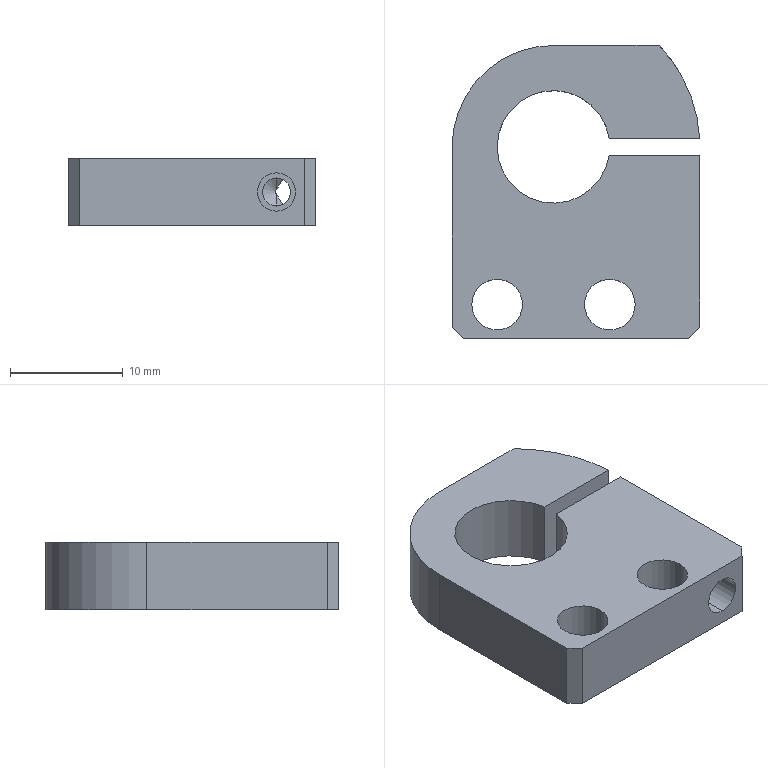Part | STEP file | FBDS-CS-020 | 1 solid | 25 faces | box 22 x 26 x 6 mm | volume 2342 mm3 | cylinder 12 | plane 10 | cone 3 | commonest cylinder face diameters 4.5 x4 2.5 x2 3.4 x2 10 x2 18 x1 26 x1
STEP:
#1=CARTESIAN_POINT('',(-581.954,-3556.136,6.));
#2=VERTEX_POINT('',#1);
#3=CARTESIAN_POINT('',(-577.454,-3556.136,6.));
#4=VERTEX_POINT('',#3);
#5=CARTESIAN_POINT('',(-579.704,-3556.136,6.));
#6=DIRECTION('',(0.,0.,1.));
#7=DIRECTION('',(1.,0.,0.));
#8=AXIS2_PLACEMENT_3D('',#5,#6,#7);
#9=CIRCLE('',#8,2.25);
#10=EDGE_CURVE('',#2,#4,#9,.T.);
#11=ORIENTED_EDGE('',*,*,#10,.T.);
#12=CARTESIAN_POINT('',(-577.454,-3556.136,0.));
#13=VERTEX_POINT('',#12);
#14=CARTESIAN_POINT('',(-577.454,-3556.136,0.));
#15=DIRECTION('',(0.,0.,-1.));
#16=VECTOR('',#15,1000.);
#17=LINE('',#14,#16);
#18=EDGE_CURVE('',#4,#13,#17,.T.);
#19=ORIENTED_EDGE('',*,*,#18,.T.);
#20=CARTESIAN_POINT('',(-581.954,-3556.136,0.));
#21=VERTEX_POINT('',#20);
#22=CARTESIAN_POINT('',(-579.704,-3556.136,0.));
#23=DIRECTION('',(0.,0.,-1.));
#24=DIRECTION('',(-1.,0.,0.));
#25=AXIS2_PLACEMENT_3D('',#22,#23,#24);
#26=CIRCLE('',#25,2.25);
#27=EDGE_CURVE('',#13,#21,#26,.T.);
#28=ORIENTED_EDGE('',*,*,#27,.T.);
#29=CARTESIAN_POINT('',(-581.954,-3556.136,0.));
#30=DIRECTION('',(0.,0.,-1.));
#31=VECTOR('',#30,1000.);
#32=LINE('',#29,#31);
#33=EDGE_CURVE('',#2,#21,#32,.T.);
#34=ORIENTED_EDGE('',*,*,#33,.F.);
#35=EDGE_LOOP('',(#11,#19,#28,#34));
#36=FACE_OUTER_BOUND('',#35,.T.);
#37=CARTESIAN_POINT('',(-579.704,-3556.136,0.));
#38=DIRECTION('',(0.,0.,-1.));
#39=DIRECTION('',(-1.,0.,0.));
#40=AXIS2_PLACEMENT_3D('',#37,#38,#39);
#41=CYLINDRICAL_SURFACE('',#40,2.25);
#42=ADVANCED_FACE('',(#36),#41,.F.);
#43=CARTESIAN_POINT('',(-591.954,-3556.136,6.));
#44=VERTEX_POINT('',#43);
#45=CARTESIAN_POINT('',(-587.454,-3556.136,6.));
#46=VERTEX_POINT('',#45);
#47=CARTESIAN_POINT('',(-589.704,-3556.136,6.));
#48=DIRECTION('',(0.,0.,1.));
#49=DIRECTION('',(1.,0.,0.));
#50=AXIS2_PLACEMENT_3D('',#47,#48,#49);
#51=CIRCLE('',#50,2.25);
#52=EDGE_CURVE('',#44,#46,#51,.T.);
#53=ORIENTED_EDGE('',*,*,#52,.T.);
#54=CARTESIAN_POINT('',(-587.454,-3556.136,0.));
#55=VERTEX_POINT('',#54);
#56=CARTESIAN_POINT('',(-587.454,-3556.136,0.));
#57=DIRECTION('',(0.,0.,-1.));
#58=VECTOR('',#57,1000.);
#59=LINE('',#56,#58);
#60=EDGE_CURVE('',#46,#55,#59,.T.);
#61=ORIENTED_EDGE('',*,*,#60,.T.);
#62=CARTESIAN_POINT('',(-591.954,-3556.136,0.));
#63=VERTEX_POINT('',#62);
#64=CARTESIAN_POINT('',(-589.704,-3556.136,0.));
#65=DIRECTION('',(0.,0.,-1.));
#66=DIRECTION('',(-1.,0.,0.));
#67=AXIS2_PLACEMENT_3D('',#64,#65,#66);
#68=CIRCLE('',#67,2.25);
#69=EDGE_CURVE('',#55,#63,#68,.T.);
#70=ORIENTED_EDGE('',*,*,#69,.T.);
#71=CARTESIAN_POINT('',(-591.954,-3556.136,0.));
#72=DIRECTION('',(0.,0.,-1.));
#73=VECTOR('',#72,1000.);
#74=LINE('',#71,#73);
#75=EDGE_CURVE('',#44,#63,#74,.T.);
#76=ORIENTED_EDGE('',*,*,#75,.F.);
#77=EDGE_LOOP('',(#53,#61,#70,#76));
#78=FACE_OUTER_BOUND('',#77,.T.);
#79=CARTESIAN_POINT('',(-589.704,-3556.136,0.));
#80=DIRECTION('',(0.,0.,-1.));
#81=DIRECTION('',(-1.,0.,0.));
#82=AXIS2_PLACEMENT_3D('',#79,#80,#81);
#83=CYLINDRICAL_SURFACE('',#82,2.25);
#84=ADVANCED_FACE('',(#78),#83,.F.);
#85=CARTESIAN_POINT('',(-575.204,-3533.262,3.211));
#86=VERTEX_POINT('',#85);
#87=CARTESIAN_POINT('',(-575.204,-3533.262,2.789));
#88=VERTEX_POINT('',#87);
#89=CARTESIAN_POINT('',(-575.204,-3533.262,3.211));
#90=CARTESIAN_POINT('',(-575.222,-3533.243,3.18));
#91=CARTESIAN_POINT('',(-575.239,-3533.225,3.148));
#92=CARTESIAN_POINT('',(-575.268,-3533.194,3.079));
#93=CARTESIAN_POINT('',(-575.28,-3533.181,3.04));
#94=CARTESIAN_POINT('',(-575.28,-3533.181,2.959));
#95=CARTESIAN_POINT('',(-575.268,-3533.194,2.92));
#96=CARTESIAN_POINT('',(-575.238,-3533.225,2.851));
#97=CARTESIAN_POINT('',(-575.221,-3533.243,2.82));
#98=CARTESIAN_POINT('',(-575.204,-3533.262,2.789));
#99=B_SPLINE_CURVE_WITH_KNOTS('',3,(#89,#90,#91,#92,#93,#94,#95,#96,#97,#98),.UNSPECIFIED.,.F.,.F.,(4,2,2,2,4),(0.00138,0.001502,0.001624,0.001746,0.001868),.UNSPECIFIED.);
#100=EDGE_CURVE('',#86,#88,#99,.T.);
#101=ORIENTED_EDGE('',*,*,#100,.F.);
#102=CARTESIAN_POINT('',(-575.204,-3533.886,4.25));
#103=VERTEX_POINT('',#102);
#104=CARTESIAN_POINT('',(-575.204,-3533.886,4.25));
#105=DIRECTION('',(0.,-0.515,0.8572));
#106=VECTOR('',#105,1000.);
#107=LINE('',#104,#106);
#108=EDGE_CURVE('',#86,#103,#107,.T.);
#109=ORIENTED_EDGE('',*,*,#108,.T.);
#110=CARTESIAN_POINT('',(-575.204,-3533.886,1.75));
#111=VERTEX_POINT('',#110);
#112=CARTESIAN_POINT('',(-575.204,-3533.886,3.));
#113=DIRECTION('',(0.,-1.,0.));
#114=DIRECTION('',(0.,0.,-1.));
#115=AXIS2_PLACEMENT_3D('',#112,#113,#114);
#116=CIRCLE('',#115,1.25);
#117=EDGE_CURVE('',#103,#111,#116,.T.);
#118=ORIENTED_EDGE('',*,*,#117,.T.);
#119=CARTESIAN_POINT('',(-575.204,-3533.886,1.75));
#120=DIRECTION('',(0.,-0.515,-0.8572));
#121=VECTOR('',#120,1000.);
#122=LINE('',#119,#121);
#123=EDGE_CURVE('',#88,#111,#122,.T.);
#124=ORIENTED_EDGE('',*,*,#123,.F.);
#125=EDGE_LOOP('',(#101,#109,#118,#124));
#126=FACE_OUTER_BOUND('',#125,.T.);
#127=CARTESIAN_POINT('',(-575.204,-3533.886,3.));
#128=DIRECTION('',(0.,-1.,0.));
#129=DIRECTION('',(0.,0.,-1.));
#130=AXIS2_PLACEMENT_3D('',#127,#128,#129);
#131=CONICAL_SURFACE('',#130,1.25,1.03);
#132=ADVANCED_FACE('',(#126),#131,.F.);
#133=CARTESIAN_POINT('',(-574.657,-3533.886,1.876));
#134=VERTEX_POINT('',#133);
#135=CARTESIAN_POINT('',(-575.204,-3533.262,2.789));
#136=CARTESIAN_POINT('',(-575.159,-3533.31,2.709));
#137=CARTESIAN_POINT('',(-575.112,-3533.362,2.634));
#138=CARTESIAN_POINT('',(-575.018,-3533.465,2.483));
#139=CARTESIAN_POINT('',(-574.972,-3533.517,2.408));
#140=CARTESIAN_POINT('',(-574.834,-3533.675,2.181));
#141=CARTESIAN_POINT('',(-574.744,-3533.781,2.029));
#142=CARTESIAN_POINT('',(-574.657,-3533.886,1.876));
#143=B_SPLINE_CURVE_WITH_KNOTS('',3,(#135,#136,#137,#138,#139,#140,#141,#142),.UNSPECIFIED.,.F.,.F.,(4,2,2,4),(0.001868,0.002179,0.00249,0.003112),.UNSPECIFIED.);
#144=EDGE_CURVE('',#88,#134,#143,.T.);
#145=ORIENTED_EDGE('',*,*,#144,.F.);
#146=ORIENTED_EDGE('',*,*,#123,.T.);
#147=CARTESIAN_POINT('',(-575.204,-3533.886,3.));
#148=DIRECTION('',(0.,-1.,0.));
#149=DIRECTION('',(0.,0.,-1.));
#150=AXIS2_PLACEMENT_3D('',#147,#148,#149);
#151=CIRCLE('',#150,1.25);
#152=EDGE_CURVE('',#111,#134,#151,.T.);
#153=ORIENTED_EDGE('',*,*,#152,.T.);
#154=EDGE_LOOP('',(#145,#146,#153));
#155=FACE_OUTER_BOUND('',#154,.T.);
#156=CARTESIAN_POINT('',(-575.204,-3533.886,3.));
#157=DIRECTION('',(0.,-1.,0.));
#158=DIRECTION('',(0.,0.,-1.));
#159=AXIS2_PLACEMENT_3D('',#156,#157,#158);
#160=CONICAL_SURFACE('',#159,1.25,1.03);
#161=ADVANCED_FACE('',(#155),#160,.F.);
#162=ORIENTED_EDGE('',*,*,#117,.F.);
#163=CARTESIAN_POINT('',(-575.204,-3541.386,4.25));
#164=VERTEX_POINT('',#163);
#165=CARTESIAN_POINT('',(-575.204,-3541.386,4.25));
#166=DIRECTION('',(0.,-1.,0.));
#167=VECTOR('',#166,1000.);
#168=LINE('',#165,#167);
#169=EDGE_CURVE('',#103,#164,#168,.T.);
#170=ORIENTED_EDGE('',*,*,#169,.T.);
#171=CARTESIAN_POINT('',(-575.204,-3541.386,1.75));
#172=VERTEX_POINT('',#171);
#173=CARTESIAN_POINT('',(-575.204,-3541.386,3.));
#174=DIRECTION('',(0.,-1.,0.));
#175=DIRECTION('',(0.,0.,-1.));
#176=AXIS2_PLACEMENT_3D('',#173,#174,#175);
#177=CIRCLE('',#176,1.25);
#178=EDGE_CURVE('',#164,#172,#177,.T.);
#179=ORIENTED_EDGE('',*,*,#178,.T.);
#180=CARTESIAN_POINT('',(-575.204,-3541.386,1.75));
#181=DIRECTION('',(0.,-1.,0.));
#182=VECTOR('',#181,1000.);
#183=LINE('',#180,#182);
#184=EDGE_CURVE('',#111,#172,#183,.T.);
#185=ORIENTED_EDGE('',*,*,#184,.F.);
#186=EDGE_LOOP('',(#162,#170,#179,#185));
#187=FACE_OUTER_BOUND('',#186,.T.);
#188=CARTESIAN_POINT('',(-575.204,-3541.386,3.));
#189=DIRECTION('',(0.,-1.,0.));
#190=DIRECTION('',(0.,0.,-1.));
#191=AXIS2_PLACEMENT_3D('',#188,#189,#190);
#192=CYLINDRICAL_SURFACE('',#191,1.25);
#193=ADVANCED_FACE('',(#187),#192,.F.);
#194=CARTESIAN_POINT('',(-575.204,-3542.886,1.3));
#195=VERTEX_POINT('',#194);
#196=CARTESIAN_POINT('',(-575.204,-3542.886,4.7));
#197=VERTEX_POINT('',#196);
#198=CARTESIAN_POINT('',(-575.204,-3542.886,3.));
#199=DIRECTION('',(0.,1.,0.));
#200=DIRECTION('',(0.,0.,-1.));
#201=AXIS2_PLACEMENT_3D('',#198,#199,#200);
#202=CIRCLE('',#201,1.7);
#203=EDGE_CURVE('',#195,#197,#202,.T.);
#204=ORIENTED_EDGE('',*,*,#203,.T.);
#205=CARTESIAN_POINT('',(-575.204,-3559.136,4.7));
#206=VERTEX_POINT('',#205);
#207=CARTESIAN_POINT('',(-575.204,-3559.136,4.7));
#208=DIRECTION('',(0.,-1.,0.));
#209=VECTOR('',#208,1000.);
#210=LINE('',#207,#209);
#211=EDGE_CURVE('',#197,#206,#210,.T.);
#212=ORIENTED_EDGE('',*,*,#211,.T.);
#213=CARTESIAN_POINT('',(-575.204,-3559.136,1.3));
#214=VERTEX_POINT('',#213);
#215=CARTESIAN_POINT('',(-575.204,-3559.136,3.));
#216=DIRECTION('',(0.,-1.,0.));
#217=DIRECTION('',(0.,0.,-1.));
#218=AXIS2_PLACEMENT_3D('',#215,#216,#217);
#219=CIRCLE('',#218,1.7);
#220=EDGE_CURVE('',#206,#214,#219,.T.);
#221=ORIENTED_EDGE('',*,*,#220,.T.);
#222=CARTESIAN_POINT('',(-575.204,-3559.136,1.3));
#223=DIRECTION('',(0.,-1.,0.));
#224=VECTOR('',#223,1000.);
#225=LINE('',#222,#224);
#226=EDGE_CURVE('',#195,#214,#225,.T.);
#227=ORIENTED_EDGE('',*,*,#226,.F.);
#228=EDGE_LOOP('',(#204,#212,#221,#227));
#229=FACE_OUTER_BOUND('',#228,.T.);
#230=CARTESIAN_POINT('',(-575.204,-3559.136,3.));
#231=DIRECTION('',(0.,-1.,0.));
#232=DIRECTION('',(0.,0.,-1.));
#233=AXIS2_PLACEMENT_3D('',#230,#231,#232);
#234=CYLINDRICAL_SURFACE('',#233,1.7);
#235=ADVANCED_FACE('',(#229),#234,.F.);
#236=CARTESIAN_POINT('',(-579.761,-3541.386,6.));
#237=VERTEX_POINT('',#236);
#238=CARTESIAN_POINT('',(-589.704,-3542.136,6.));
#239=VERTEX_POINT('',#238);
#240=CARTESIAN_POINT('',(-584.704,-3542.136,6.));
#241=DIRECTION('',(0.,0.,1.));
#242=DIRECTION('',(1.,0.,0.));
#243=AXIS2_PLACEMENT_3D('',#240,#241,#242);
#244=CIRCLE('',#243,5.);
#245=EDGE_CURVE('',#237,#239,#244,.T.);
#246=ORIENTED_EDGE('',*,*,#245,.T.);
#247=CARTESIAN_POINT('',(-589.704,-3542.136,0.));
#248=VERTEX_POINT('',#247);
#249=CARTESIAN_POINT('',(-589.704,-3542.136,6.));
#250=DIRECTION('',(0.,0.,-1.));
#251=VECTOR('',#250,1000.);
#252=LINE('',#249,#251);
#253=EDGE_CURVE('',#239,#248,#252,.T.);
#254=ORIENTED_EDGE('',*,*,#253,.T.);
#255=CARTESIAN_POINT('',(-579.761,-3541.386,0.));
#256=VERTEX_POINT('',#255);
#257=CARTESIAN_POINT('',(-584.704,-3542.136,0.));
#258=DIRECTION('',(0.,0.,1.));
#259=DIRECTION('',(1.,0.,0.));
#260=AXIS2_PLACEMENT_3D('',#257,#258,#259);
#261=CIRCLE('',#260,5.);
#262=EDGE_CURVE('',#256,#248,#261,.T.);
#263=ORIENTED_EDGE('',*,*,#262,.F.);
#264=CARTESIAN_POINT('',(-579.761,-3541.386,6.));
#265=DIRECTION('',(0.,0.,-1.));
#266=VECTOR('',#265,1000.);
#267=LINE('',#264,#266);
#268=EDGE_CURVE('',#237,#256,#267,.T.);
#269=ORIENTED_EDGE('',*,*,#268,.F.);
#270=EDGE_LOOP('',(#246,#254,#263,#269));
#271=FACE_OUTER_BOUND('',#270,.T.);
#272=CARTESIAN_POINT('',(-584.704,-3542.136,6.));
#273=DIRECTION('',(0.,0.,-1.));
#274=DIRECTION('',(-1.,0.,0.));
#275=AXIS2_PLACEMENT_3D('',#272,#273,#274);
#276=CYLINDRICAL_SURFACE('',#275,5.);
#277=ADVANCED_FACE('',(#271),#276,.F.);
#278=CARTESIAN_POINT('',(-593.704,-3558.136,6.));
#279=VERTEX_POINT('',#278);
#280=CARTESIAN_POINT('',(-593.704,-3542.136,6.));
#281=VERTEX_POINT('',#280);
#282=CARTESIAN_POINT('',(-593.704,-3542.136,6.));
#283=DIRECTION('',(0.,1.,0.));
#284=VECTOR('',#283,1000.);
#285=LINE('',#282,#284);
#286=EDGE_CURVE('',#279,#281,#285,.T.);
#287=ORIENTED_EDGE('',*,*,#286,.F.);
#288=CARTESIAN_POINT('',(-592.704,-3559.136,6.));
#289=VERTEX_POINT('',#288);
#290=CARTESIAN_POINT('',(-597.204,-3554.636,6.));
#291=DIRECTION('',(0.7071,-0.7071,0.));
#292=VECTOR('',#291,1000.);
#293=LINE('',#290,#292);
#294=EDGE_CURVE('',#279,#289,#293,.T.);
#295=ORIENTED_EDGE('',*,*,#294,.T.);
#296=CARTESIAN_POINT('',(-572.704,-3559.136,6.));
#297=VERTEX_POINT('',#296);
#298=CARTESIAN_POINT('',(-597.704,-3559.136,6.));
#299=DIRECTION('',(1.,0.,0.));
#300=VECTOR('',#299,1000.);
#301=LINE('',#298,#300);
#302=EDGE_CURVE('',#289,#297,#301,.T.);
#303=ORIENTED_EDGE('',*,*,#302,.T.);
#304=CARTESIAN_POINT('',(-571.704,-3558.136,6.));
#305=VERTEX_POINT('',#304);
#306=CARTESIAN_POINT('',(-570.204,-3556.636,6.));
#307=DIRECTION('',(0.7071,0.7071,0.));
#308=VECTOR('',#307,1000.);
#309=LINE('',#306,#308);
#310=EDGE_CURVE('',#297,#305,#309,.T.);
#311=ORIENTED_EDGE('',*,*,#310,.T.);
#312=CARTESIAN_POINT('',(-571.704,-3542.886,6.));
#313=VERTEX_POINT('',#312);
#314=CARTESIAN_POINT('',(-571.704,-3542.136,6.));
#315=DIRECTION('',(0.,1.,0.));
#316=VECTOR('',#315,1000.);
#317=LINE('',#314,#316);
#318=EDGE_CURVE('',#305,#313,#317,.T.);
#319=ORIENTED_EDGE('',*,*,#318,.T.);
#320=CARTESIAN_POINT('',(-579.761,-3542.886,6.));
#321=VERTEX_POINT('',#320);
#322=CARTESIAN_POINT('',(-580.24,-3542.886,6.));
#323=DIRECTION('',(1.,0.,0.));
#324=VECTOR('',#323,1000.);
#325=LINE('',#322,#324);
#326=EDGE_CURVE('',#321,#313,#325,.T.);
#327=ORIENTED_EDGE('',*,*,#326,.F.);
#328=CARTESIAN_POINT('',(-584.704,-3542.136,6.));
#329=DIRECTION('',(0.,0.,1.));
#330=DIRECTION('',(1.,0.,0.));
#331=AXIS2_PLACEMENT_3D('',#328,#329,#330);
#332=CIRCLE('',#331,5.);
#333=EDGE_CURVE('',#239,#321,#332,.T.);
#334=ORIENTED_EDGE('',*,*,#333,.F.);
#335=ORIENTED_EDGE('',*,*,#245,.F.);
#336=CARTESIAN_POINT('',(-571.726,-3541.386,6.));
#337=VERTEX_POINT('',#336);
#338=CARTESIAN_POINT('',(-580.24,-3541.386,6.));
#339=DIRECTION('',(-1.,0.,0.));
#340=VECTOR('',#339,1000.);
#341=LINE('',#338,#340);
#342=EDGE_CURVE('',#337,#237,#341,.T.);
#343=ORIENTED_EDGE('',*,*,#342,.F.);
#344=CARTESIAN_POINT('',(-575.323,-3533.136,6.));
#345=VERTEX_POINT('',#344);
#346=CARTESIAN_POINT('',(-584.704,-3542.136,6.));
#347=DIRECTION('',(0.,0.,1.));
#348=DIRECTION('',(1.,0.,0.));
#349=AXIS2_PLACEMENT_3D('',#346,#347,#348);
#350=CIRCLE('',#349,13.);
#351=EDGE_CURVE('',#337,#345,#350,.T.);
#352=ORIENTED_EDGE('',*,*,#351,.T.);
#353=CARTESIAN_POINT('',(-584.704,-3533.136,6.));
#354=VERTEX_POINT('',#353);
#355=CARTESIAN_POINT('',(-584.704,-3533.136,6.));
#356=DIRECTION('',(1.,0.,0.));
#357=VECTOR('',#356,1000.);
#358=LINE('',#355,#357);
#359=EDGE_CURVE('',#354,#345,#358,.T.);
#360=ORIENTED_EDGE('',*,*,#359,.F.);
#361=CARTESIAN_POINT('',(-584.704,-3542.136,6.));
#362=DIRECTION('',(0.,0.,-1.));
#363=DIRECTION('',(1.,0.,0.));
#364=AXIS2_PLACEMENT_3D('',#361,#362,#363);
#365=CIRCLE('',#364,9.);
#366=EDGE_CURVE('',#281,#354,#365,.T.);
#367=ORIENTED_EDGE('',*,*,#366,.F.);
#368=EDGE_LOOP('',(#287,#295,#303,#311,#319,#327,#334,#335,#343,#352,#360,#367));
#369=FACE_OUTER_BOUND('',#368,.T.);
#370=ORIENTED_EDGE('',*,*,#10,.F.);
#371=CARTESIAN_POINT('',(-579.704,-3556.136,6.));
#372=DIRECTION('',(0.,0.,1.));
#373=DIRECTION('',(1.,0.,0.));
#374=AXIS2_PLACEMENT_3D('',#371,#372,#373);
#375=CIRCLE('',#374,2.25);
#376=EDGE_CURVE('',#4,#2,#375,.T.);
#377=ORIENTED_EDGE('',*,*,#376,.F.);
#378=EDGE_LOOP('',(#370,#377));
#379=FACE_BOUND('',#378,.T.);
#380=ORIENTED_EDGE('',*,*,#52,.F.);
#381=CARTESIAN_POINT('',(-589.704,-3556.136,6.));
#382=DIRECTION('',(0.,0.,1.));
#383=DIRECTION('',(1.,0.,0.));
#384=AXIS2_PLACEMENT_3D('',#381,#382,#383);
#385=CIRCLE('',#384,2.25);
#386=EDGE_CURVE('',#46,#44,#385,.T.);
#387=ORIENTED_EDGE('',*,*,#386,.F.);
#388=EDGE_LOOP('',(#380,#387));
#389=FACE_BOUND('',#388,.T.);
#390=CARTESIAN_POINT('',(-584.704,-3542.136,6.));
#391=DIRECTION('',(0.,0.,1.));
#392=DIRECTION('',(1.,0.,0.));
#393=AXIS2_PLACEMENT_3D('',#390,#391,#392);
#394=PLANE('',#393);
#395=ADVANCED_FACE('',(#369,#379,#389),#394,.T.);
#396=CARTESIAN_POINT('',(-579.704,-3556.136,0.));
#397=DIRECTION('',(0.,0.,-1.));
#398=DIRECTION('',(-1.,0.,0.));
#399=AXIS2_PLACEMENT_3D('',#396,#397,#398);
#400=CIRCLE('',#399,2.25);
#401=EDGE_CURVE('',#21,#13,#400,.T.);
#402=ORIENTED_EDGE('',*,*,#401,.F.);
#403=ORIENTED_EDGE('',*,*,#27,.F.);
#404=EDGE_LOOP('',(#402,#403));
#405=FACE_BOUND('',#404,.T.);
#406=CARTESIAN_POINT('',(-589.704,-3556.136,0.));
#407=DIRECTION('',(0.,0.,-1.));
#408=DIRECTION('',(-1.,0.,0.));
#409=AXIS2_PLACEMENT_3D('',#406,#407,#408);
#410=CIRCLE('',#409,2.25);
#411=EDGE_CURVE('',#63,#55,#410,.T.);
#412=ORIENTED_EDGE('',*,*,#411,.F.);
#413=ORIENTED_EDGE('',*,*,#69,.F.);
#414=EDGE_LOOP('',(#412,#413));
#415=FACE_BOUND('',#414,.T.);
#416=CARTESIAN_POINT('',(-592.704,-3559.136,0.));
#417=VERTEX_POINT('',#416);
#418=CARTESIAN_POINT('',(-572.704,-3559.136,0.));
#419=VERTEX_POINT('',#418);
#420=CARTESIAN_POINT('',(-597.704,-3559.136,0.));
#421=DIRECTION('',(1.,0.,0.));
#422=VECTOR('',#421,1000.);
#423=LINE('',#420,#422);
#424=EDGE_CURVE('',#417,#419,#423,.T.);
#425=ORIENTED_EDGE('',*,*,#424,.F.);
#426=CARTESIAN_POINT('',(-593.704,-3558.136,0.));
#427=VERTEX_POINT('',#426);
#428=CARTESIAN_POINT('',(-592.704,-3559.136,0.));
#429=DIRECTION('',(-0.7071,0.7071,0.));
#430=VECTOR('',#429,1000.);
#431=LINE('',#428,#430);
#432=EDGE_CURVE('',#417,#427,#431,.T.);
#433=ORIENTED_EDGE('',*,*,#432,.T.);
#434=CARTESIAN_POINT('',(-593.704,-3542.136,0.));
#435=VERTEX_POINT('',#434);
#436=CARTESIAN_POINT('',(-593.704,-3542.136,0.));
#437=DIRECTION('',(0.,1.,0.));
#438=VECTOR('',#437,1000.);
#439=LINE('',#436,#438);
#440=EDGE_CURVE('',#427,#435,#439,.T.);
#441=ORIENTED_EDGE('',*,*,#440,.T.);
#442=CARTESIAN_POINT('',(-584.704,-3533.136,0.));
#443=VERTEX_POINT('',#442);
#444=CARTESIAN_POINT('',(-584.704,-3542.136,0.));
#445=DIRECTION('',(0.,0.,-1.));
#446=DIRECTION('',(1.,0.,0.));
#447=AXIS2_PLACEMENT_3D('',#444,#445,#446);
#448=CIRCLE('',#447,9.);
#449=EDGE_CURVE('',#435,#443,#448,.T.);
#450=ORIENTED_EDGE('',*,*,#449,.T.);
#451=CARTESIAN_POINT('',(-575.323,-3533.136,0.));
#452=VERTEX_POINT('',#451);
#453=CARTESIAN_POINT('',(-584.704,-3533.136,0.));
#454=DIRECTION('',(1.,0.,0.));
#455=VECTOR('',#454,1000.);
#456=LINE('',#453,#455);
#457=EDGE_CURVE('',#443,#452,#456,.T.);
#458=ORIENTED_EDGE('',*,*,#457,.T.);
#459=CARTESIAN_POINT('',(-571.726,-3541.386,0.));
#460=VERTEX_POINT('',#459);
#461=CARTESIAN_POINT('',(-584.704,-3542.136,0.));
#462=DIRECTION('',(0.,0.,1.));
#463=DIRECTION('',(1.,0.,0.));
#464=AXIS2_PLACEMENT_3D('',#461,#462,#463);
#465=CIRCLE('',#464,13.);
#466=EDGE_CURVE('',#460,#452,#465,.T.);
#467=ORIENTED_EDGE('',*,*,#466,.F.);
#468=CARTESIAN_POINT('',(-580.24,-3541.386,0.));
#469=DIRECTION('',(-1.,0.,0.));
#470=VECTOR('',#469,1000.);
#471=LINE('',#468,#470);
#472=EDGE_CURVE('',#460,#256,#471,.T.);
#473=ORIENTED_EDGE('',*,*,#472,.T.);
#474=ORIENTED_EDGE('',*,*,#262,.T.);
#475=CARTESIAN_POINT('',(-579.761,-3542.886,0.));
#476=VERTEX_POINT('',#475);
#477=CARTESIAN_POINT('',(-584.704,-3542.136,0.));
#478=DIRECTION('',(0.,0.,1.));
#479=DIRECTION('',(1.,0.,0.));
#480=AXIS2_PLACEMENT_3D('',#477,#478,#479);
#481=CIRCLE('',#480,5.);
#482=EDGE_CURVE('',#248,#476,#481,.T.);
#483=ORIENTED_EDGE('',*,*,#482,.T.);
#484=CARTESIAN_POINT('',(-571.704,-3542.886,0.));
#485=VERTEX_POINT('',#484);
#486=CARTESIAN_POINT('',(-580.24,-3542.886,0.));
#487=DIRECTION('',(1.,0.,0.));
#488=VECTOR('',#487,1000.);
#489=LINE('',#486,#488);
#490=EDGE_CURVE('',#476,#485,#489,.T.);
#491=ORIENTED_EDGE('',*,*,#490,.T.);
#492=CARTESIAN_POINT('',(-571.704,-3558.136,0.));
#493=VERTEX_POINT('',#492);
#494=CARTESIAN_POINT('',(-571.704,-3542.136,0.));
#495=DIRECTION('',(0.,1.,0.));
#496=VECTOR('',#495,1000.);
#497=LINE('',#494,#496);
#498=EDGE_CURVE('',#493,#485,#497,.T.);
#499=ORIENTED_EDGE('',*,*,#498,.F.);
#500=CARTESIAN_POINT('',(-571.704,-3558.136,0.));
#501=DIRECTION('',(-0.7071,-0.7071,0.));
#502=VECTOR('',#501,1000.);
#503=LINE('',#500,#502);
#504=EDGE_CURVE('',#493,#419,#503,.T.);
#505=ORIENTED_EDGE('',*,*,#504,.T.);
#506=EDGE_LOOP('',(#425,#433,#441,#450,#458,#467,#473,#474,#483,#491,#499,#505));
#507=FACE_OUTER_BOUND('',#506,.T.);
#508=CARTESIAN_POINT('',(-584.704,-3542.136,0.));
#509=DIRECTION('',(0.,0.,1.));
#510=DIRECTION('',(1.,0.,0.));
#511=AXIS2_PLACEMENT_3D('',#508,#509,#510);
#512=PLANE('',#511);
#513=ADVANCED_FACE('',(#405,#415,#507),#512,.F.);
#514=CARTESIAN_POINT('',(-574.657,-3533.886,4.124));
#515=VERTEX_POINT('',#514);
#516=CARTESIAN_POINT('',(-574.657,-3533.886,4.124));
#517=CARTESIAN_POINT('',(-574.744,-3533.781,3.971));
#518=CARTESIAN_POINT('',(-574.834,-3533.675,3.819));
#519=CARTESIAN_POINT('',(-574.972,-3533.517,3.592));
#520=CARTESIAN_POINT('',(-575.018,-3533.465,3.517));
#521=CARTESIAN_POINT('',(-575.112,-3533.362,3.366));
#522=CARTESIAN_POINT('',(-575.159,-3533.31,3.291));
#523=CARTESIAN_POINT('',(-575.204,-3533.262,3.211));
#524=B_SPLINE_CURVE_WITH_KNOTS('',3,(#516,#517,#518,#519,#520,#521,#522,#523),.UNSPECIFIED.,.F.,.F.,(4,2,2,4),(0.0001464,0.0007632,0.001072,0.00138),.UNSPECIFIED.);
#525=EDGE_CURVE('',#515,#86,#524,.T.);
#526=ORIENTED_EDGE('',*,*,#525,.T.);
#527=ORIENTED_EDGE('',*,*,#100,.T.);
#528=ORIENTED_EDGE('',*,*,#144,.T.);
#529=CARTESIAN_POINT('',(-574.657,-3533.886,1.876));
#530=CARTESIAN_POINT('',(-574.57,-3533.993,1.919));
#531=CARTESIAN_POINT('',(-574.487,-3534.097,1.971));
#532=CARTESIAN_POINT('',(-574.331,-3534.299,2.099));
#533=CARTESIAN_POINT('',(-574.258,-3534.397,2.175));
#534=CARTESIAN_POINT('',(-574.126,-3534.579,2.358));
#535=CARTESIAN_POINT('',(-574.067,-3534.662,2.465));
#536=CARTESIAN_POINT('',(-573.981,-3534.786,2.709));
#537=CARTESIAN_POINT('',(-573.954,-3534.826,2.851));
#538=CARTESIAN_POINT('',(-573.954,-3534.827,3.141));
#539=CARTESIAN_POINT('',(-573.98,-3534.788,3.285));
#540=CARTESIAN_POINT('',(-574.065,-3534.665,3.532));
#541=CARTESIAN_POINT('',(-574.124,-3534.582,3.639));
#542=CARTESIAN_POINT('',(-574.255,-3534.402,3.821));
#543=CARTESIAN_POINT('',(-574.329,-3534.302,3.898));
#544=CARTESIAN_POINT('',(-574.486,-3534.098,4.028));
#545=CARTESIAN_POINT('',(-574.569,-3533.993,4.081));
#546=CARTESIAN_POINT('',(-574.657,-3533.886,4.124));
#547=B_SPLINE_CURVE_WITH_KNOTS('',3,(#529,#530,#531,#532,#533,#534,#535,#536,#537,#538,#539,#540,#541,#542,#543,#544,#545,#546),.UNSPECIFIED.,.F.,.F.,(4,2,2,2,2,2,2,2,4),(0.,0.0004278,0.0008555,0.001283,0.001711,0.002139,0.002567,0.002994,0.003422),.UNSPECIFIED.);
#548=EDGE_CURVE('',#134,#515,#547,.T.);
#549=ORIENTED_EDGE('',*,*,#548,.T.);
#550=EDGE_LOOP('',(#526,#527,#528,#549));
#551=FACE_BOUND('',#550,.T.);
#552=ORIENTED_EDGE('',*,*,#466,.T.);
#553=CARTESIAN_POINT('',(-575.323,-3533.136,-4.));
#554=DIRECTION('',(0.,0.,1.));
#555=VECTOR('',#554,1000.);
#556=LINE('',#553,#555);
#557=EDGE_CURVE('',#452,#345,#556,.T.);
#558=ORIENTED_EDGE('',*,*,#557,.T.);
#559=ORIENTED_EDGE('',*,*,#351,.F.);
#560=CARTESIAN_POINT('',(-571.726,-3541.386,6.));
#561=DIRECTION('',(0.,0.,-1.));
#562=VECTOR('',#561,1000.);
#563=LINE('',#560,#562);
#564=EDGE_CURVE('',#337,#460,#563,.T.);
#565=ORIENTED_EDGE('',*,*,#564,.T.);
#566=EDGE_LOOP('',(#552,#558,#559,#565));
#567=FACE_OUTER_BOUND('',#566,.T.);
#568=CARTESIAN_POINT('',(-584.704,-3542.136,6.));
#569=DIRECTION('',(0.,0.,-1.));
#570=DIRECTION('',(-1.,0.,0.));
#571=AXIS2_PLACEMENT_3D('',#568,#569,#570);
#572=CYLINDRICAL_SURFACE('',#571,13.);
#573=ADVANCED_FACE('',(#551,#567),#572,.T.);
#574=CARTESIAN_POINT('',(-575.204,-3559.136,3.));
#575=DIRECTION('',(0.,-1.,0.));
#576=DIRECTION('',(0.,0.,-1.));
#577=AXIS2_PLACEMENT_3D('',#574,#575,#576);
#578=CIRCLE('',#577,1.7);
#579=EDGE_CURVE('',#214,#206,#578,.T.);
#580=ORIENTED_EDGE('',*,*,#579,.F.);
#581=ORIENTED_EDGE('',*,*,#220,.F.);
#582=EDGE_LOOP('',(#580,#581));
#583=FACE_BOUND('',#582,.T.);
#584=ORIENTED_EDGE('',*,*,#302,.F.);
#585=CARTESIAN_POINT('',(-592.704,-3559.136,6.));
#586=DIRECTION('',(0.,0.,-1.));
#587=VECTOR('',#586,1000.);
#588=LINE('',#585,#587);
#589=EDGE_CURVE('',#289,#417,#588,.T.);
#590=ORIENTED_EDGE('',*,*,#589,.T.);
#591=ORIENTED_EDGE('',*,*,#424,.T.);
#592=CARTESIAN_POINT('',(-572.704,-3559.136,6.));
#593=DIRECTION('',(0.,0.,1.));
#594=VECTOR('',#593,1000.);
#595=LINE('',#592,#594);
#596=EDGE_CURVE('',#419,#297,#595,.T.);
#597=ORIENTED_EDGE('',*,*,#596,.T.);
#598=EDGE_LOOP('',(#584,#590,#591,#597));
#599=FACE_OUTER_BOUND('',#598,.T.);
#600=CARTESIAN_POINT('',(-597.704,-3559.136,6.));
#601=DIRECTION('',(0.,1.,0.));
#602=DIRECTION('',(0.,0.,1.));
#603=AXIS2_PLACEMENT_3D('',#600,#601,#602);
#604=PLANE('',#603);
#605=ADVANCED_FACE('',(#583,#599),#604,.F.);
#606=ORIENTED_EDGE('',*,*,#318,.F.);
#607=CARTESIAN_POINT('',(-571.704,-3558.136,6.));
#608=DIRECTION('',(0.,0.,-1.));
#609=VECTOR('',#608,1000.);
#610=LINE('',#607,#609);
#611=EDGE_CURVE('',#305,#493,#610,.T.);
#612=ORIENTED_EDGE('',*,*,#611,.T.);
#613=ORIENTED_EDGE('',*,*,#498,.T.);
#614=CARTESIAN_POINT('',(-571.704,-3542.886,6.));
#615=DIRECTION('',(0.,0.,1.));
#616=VECTOR('',#615,1000.);
#617=LINE('',#614,#616);
#618=EDGE_CURVE('',#485,#313,#617,.T.);
#619=ORIENTED_EDGE('',*,*,#618,.T.);
#620=EDGE_LOOP('',(#606,#612,#613,#619));
#621=FACE_OUTER_BOUND('',#620,.T.);
#622=CARTESIAN_POINT('',(-571.704,-3542.136,6.));
#623=DIRECTION('',(-1.,0.,0.));
#624=DIRECTION('',(0.,0.,1.));
#625=AXIS2_PLACEMENT_3D('',#622,#623,#624);
#626=PLANE('',#625);
#627=ADVANCED_FACE('',(#621),#626,.F.);
#628=ORIENTED_EDGE('',*,*,#253,.F.);
#629=ORIENTED_EDGE('',*,*,#333,.T.);
#630=CARTESIAN_POINT('',(-579.761,-3542.886,6.));
#631=DIRECTION('',(0.,0.,1.));
#632=VECTOR('',#631,1000.);
#633=LINE('',#630,#632);
#634=EDGE_CURVE('',#476,#321,#633,.T.);
#635=ORIENTED_EDGE('',*,*,#634,.F.);
#636=ORIENTED_EDGE('',*,*,#482,.F.);
#637=EDGE_LOOP('',(#628,#629,#635,#636));
#638=FACE_OUTER_BOUND('',#637,.T.);
#639=CARTESIAN_POINT('',(-584.704,-3542.136,6.));
#640=DIRECTION('',(0.,0.,-1.));
#641=DIRECTION('',(-1.,0.,0.));
#642=AXIS2_PLACEMENT_3D('',#639,#640,#641);
#643=CYLINDRICAL_SURFACE('',#642,5.);
#644=ADVANCED_FACE('',(#638),#643,.F.);
#645=ORIENTED_EDGE('',*,*,#203,.F.);
#646=CARTESIAN_POINT('',(-575.204,-3542.886,3.));
#647=DIRECTION('',(0.,1.,0.));
#648=DIRECTION('',(0.,0.,-1.));
#649=AXIS2_PLACEMENT_3D('',#646,#647,#648);
#650=CIRCLE('',#649,1.7);
#651=EDGE_CURVE('',#197,#195,#650,.T.);
#652=ORIENTED_EDGE('',*,*,#651,.F.);
#653=EDGE_LOOP('',(#645,#652));
#654=FACE_BOUND('',#653,.T.);
#655=ORIENTED_EDGE('',*,*,#490,.F.);
#656=ORIENTED_EDGE('',*,*,#634,.T.);
#657=ORIENTED_EDGE('',*,*,#326,.T.);
#658=ORIENTED_EDGE('',*,*,#618,.F.);
#659=EDGE_LOOP('',(#655,#656,#657,#658));
#660=FACE_OUTER_BOUND('',#659,.T.);
#661=CARTESIAN_POINT('',(-580.24,-3542.886,0.));
#662=DIRECTION('',(0.,-1.,0.));
#663=DIRECTION('',(0.,0.,-1.));
#664=AXIS2_PLACEMENT_3D('',#661,#662,#663);
#665=PLANE('',#664);
#666=ADVANCED_FACE('',(#654,#660),#665,.F.);
#667=CARTESIAN_POINT('',(-575.204,-3541.386,3.));
#668=DIRECTION('',(0.,-1.,0.));
#669=DIRECTION('',(0.,0.,-1.));
#670=AXIS2_PLACEMENT_3D('',#667,#668,#669);
#671=CIRCLE('',#670,1.25);
#672=EDGE_CURVE('',#172,#164,#671,.T.);
#673=ORIENTED_EDGE('',*,*,#672,.F.);
#674=ORIENTED_EDGE('',*,*,#178,.F.);
#675=EDGE_LOOP('',(#673,#674));
#676=FACE_BOUND('',#675,.T.);
#677=ORIENTED_EDGE('',*,*,#342,.T.);
#678=ORIENTED_EDGE('',*,*,#268,.T.);
#679=ORIENTED_EDGE('',*,*,#472,.F.);
#680=ORIENTED_EDGE('',*,*,#564,.F.);
#681=EDGE_LOOP('',(#677,#678,#679,#680));
#682=FACE_OUTER_BOUND('',#681,.T.);
#683=CARTESIAN_POINT('',(-580.24,-3541.386,0.));
#684=DIRECTION('',(0.,1.,0.));
#685=DIRECTION('',(0.,0.,1.));
#686=AXIS2_PLACEMENT_3D('',#683,#684,#685);
#687=PLANE('',#686);
#688=ADVANCED_FACE('',(#676,#682),#687,.F.);
#689=ORIENTED_EDGE('',*,*,#211,.F.);
#690=ORIENTED_EDGE('',*,*,#651,.T.);
#691=ORIENTED_EDGE('',*,*,#226,.T.);
#692=ORIENTED_EDGE('',*,*,#579,.T.);
#693=EDGE_LOOP('',(#689,#690,#691,#692));
#694=FACE_OUTER_BOUND('',#693,.T.);
#695=CARTESIAN_POINT('',(-575.204,-3559.136,3.));
#696=DIRECTION('',(0.,-1.,0.));
#697=DIRECTION('',(0.,0.,-1.));
#698=AXIS2_PLACEMENT_3D('',#695,#696,#697);
#699=CYLINDRICAL_SURFACE('',#698,1.7);
#700=ADVANCED_FACE('',(#694),#699,.F.);
#701=ORIENTED_EDGE('',*,*,#169,.F.);
#702=CARTESIAN_POINT('',(-575.204,-3533.886,3.));
#703=DIRECTION('',(0.,-1.,0.));
#704=DIRECTION('',(0.,0.,-1.));
#705=AXIS2_PLACEMENT_3D('',#702,#703,#704);
#706=CIRCLE('',#705,1.25);
#707=EDGE_CURVE('',#515,#103,#706,.T.);
#708=ORIENTED_EDGE('',*,*,#707,.F.);
#709=ORIENTED_EDGE('',*,*,#548,.F.);
#710=ORIENTED_EDGE('',*,*,#152,.F.);
#711=ORIENTED_EDGE('',*,*,#184,.T.);
#712=ORIENTED_EDGE('',*,*,#672,.T.);
#713=EDGE_LOOP('',(#701,#708,#709,#710,#711,#712));
#714=FACE_OUTER_BOUND('',#713,.T.);
#715=CARTESIAN_POINT('',(-575.204,-3541.386,3.));
#716=DIRECTION('',(0.,-1.,0.));
#717=DIRECTION('',(0.,0.,-1.));
#718=AXIS2_PLACEMENT_3D('',#715,#716,#717);
#719=CYLINDRICAL_SURFACE('',#718,1.25);
#720=ADVANCED_FACE('',(#714),#719,.F.);
#721=ORIENTED_EDGE('',*,*,#108,.F.);
#722=ORIENTED_EDGE('',*,*,#525,.F.);
#723=ORIENTED_EDGE('',*,*,#707,.T.);
#724=EDGE_LOOP('',(#721,#722,#723));
#725=FACE_OUTER_BOUND('',#724,.T.);
#726=CARTESIAN_POINT('',(-575.204,-3533.886,3.));
#727=DIRECTION('',(0.,-1.,0.));
#728=DIRECTION('',(0.,0.,-1.));
#729=AXIS2_PLACEMENT_3D('',#726,#727,#728);
#730=CONICAL_SURFACE('',#729,1.25,1.03);
#731=ADVANCED_FACE('',(#725),#730,.F.);
#732=ORIENTED_EDGE('',*,*,#60,.F.);
#733=ORIENTED_EDGE('',*,*,#386,.T.);
#734=ORIENTED_EDGE('',*,*,#75,.T.);
#735=ORIENTED_EDGE('',*,*,#411,.T.);
#736=EDGE_LOOP('',(#732,#733,#734,#735));
#737=FACE_OUTER_BOUND('',#736,.T.);
#738=CARTESIAN_POINT('',(-589.704,-3556.136,0.));
#739=DIRECTION('',(0.,0.,-1.));
#740=DIRECTION('',(-1.,0.,0.));
#741=AXIS2_PLACEMENT_3D('',#738,#739,#740);
#742=CYLINDRICAL_SURFACE('',#741,2.25);
#743=ADVANCED_FACE('',(#737),#742,.F.);
#744=ORIENTED_EDGE('',*,*,#18,.F.);
#745=ORIENTED_EDGE('',*,*,#376,.T.);
#746=ORIENTED_EDGE('',*,*,#33,.T.);
#747=ORIENTED_EDGE('',*,*,#401,.T.);
#748=EDGE_LOOP('',(#744,#745,#746,#747));
#749=FACE_OUTER_BOUND('',#748,.T.);
#750=CARTESIAN_POINT('',(-579.704,-3556.136,0.));
#751=DIRECTION('',(0.,0.,-1.));
#752=DIRECTION('',(-1.,0.,0.));
#753=AXIS2_PLACEMENT_3D('',#750,#751,#752);
#754=CYLINDRICAL_SURFACE('',#753,2.25);
#755=ADVANCED_FACE('',(#749),#754,.F.);
#756=ORIENTED_EDGE('',*,*,#310,.F.);
#757=ORIENTED_EDGE('',*,*,#596,.F.);
#758=ORIENTED_EDGE('',*,*,#504,.F.);
#759=ORIENTED_EDGE('',*,*,#611,.F.);
#760=EDGE_LOOP('',(#756,#757,#758,#759));
#761=FACE_OUTER_BOUND('',#760,.T.);
#762=CARTESIAN_POINT('',(-571.704,-3558.136,6.));
#763=DIRECTION('',(-0.7071,0.7071,0.));
#764=DIRECTION('',(0.,0.,-1.));
#765=AXIS2_PLACEMENT_3D('',#762,#763,#764);
#766=PLANE('',#765);
#767=ADVANCED_FACE('',(#761),#766,.F.);
#768=CARTESIAN_POINT('',(-593.704,-3542.136,-4.));
#769=DIRECTION('',(0.,0.,1.));
#770=VECTOR('',#769,1000.);
#771=LINE('',#768,#770);
#772=EDGE_CURVE('',#435,#281,#771,.T.);
#773=ORIENTED_EDGE('',*,*,#772,.T.);
#774=ORIENTED_EDGE('',*,*,#366,.T.);
#775=CARTESIAN_POINT('',(-584.704,-3533.136,-4.));
#776=DIRECTION('',(0.,0.,1.));
#777=VECTOR('',#776,1000.);
#778=LINE('',#775,#777);
#779=EDGE_CURVE('',#443,#354,#778,.T.);
#780=ORIENTED_EDGE('',*,*,#779,.F.);
#781=ORIENTED_EDGE('',*,*,#449,.F.);
#782=EDGE_LOOP('',(#773,#774,#780,#781));
#783=FACE_OUTER_BOUND('',#782,.T.);
#784=CARTESIAN_POINT('',(-584.704,-3542.136,-4.));
#785=DIRECTION('',(0.,0.,1.));
#786=DIRECTION('',(1.,0.,0.));
#787=AXIS2_PLACEMENT_3D('',#784,#785,#786);
#788=CYLINDRICAL_SURFACE('',#787,9.);
#789=ADVANCED_FACE('',(#783),#788,.T.);
#790=ORIENTED_EDGE('',*,*,#779,.T.);
#791=ORIENTED_EDGE('',*,*,#359,.T.);
#792=ORIENTED_EDGE('',*,*,#557,.F.);
#793=ORIENTED_EDGE('',*,*,#457,.F.);
#794=EDGE_LOOP('',(#790,#791,#792,#793));
#795=FACE_OUTER_BOUND('',#794,.T.);
#796=CARTESIAN_POINT('',(-584.704,-3533.136,-4.));
#797=DIRECTION('',(0.,-1.,0.));
#798=DIRECTION('',(0.,0.,-1.));
#799=AXIS2_PLACEMENT_3D('',#796,#797,#798);
#800=PLANE('',#799);
#801=ADVANCED_FACE('',(#795),#800,.F.);
#802=ORIENTED_EDGE('',*,*,#440,.F.);
#803=CARTESIAN_POINT('',(-593.704,-3558.136,-4.));
#804=DIRECTION('',(0.,0.,1.));
#805=VECTOR('',#804,1000.);
#806=LINE('',#803,#805);
#807=EDGE_CURVE('',#427,#279,#806,.T.);
#808=ORIENTED_EDGE('',*,*,#807,.T.);
#809=ORIENTED_EDGE('',*,*,#286,.T.);
#810=ORIENTED_EDGE('',*,*,#772,.F.);
#811=EDGE_LOOP('',(#802,#808,#809,#810));
#812=FACE_OUTER_BOUND('',#811,.T.);
#813=CARTESIAN_POINT('',(-593.704,-3542.136,-4.));
#814=DIRECTION('',(1.,0.,0.));
#815=DIRECTION('',(0.,0.,-1.));
#816=AXIS2_PLACEMENT_3D('',#813,#814,#815);
#817=PLANE('',#816);
#818=ADVANCED_FACE('',(#812),#817,.F.);
#819=ORIENTED_EDGE('',*,*,#294,.F.);
#820=ORIENTED_EDGE('',*,*,#807,.F.);
#821=ORIENTED_EDGE('',*,*,#432,.F.);
#822=ORIENTED_EDGE('',*,*,#589,.F.);
#823=EDGE_LOOP('',(#819,#820,#821,#822));
#824=FACE_OUTER_BOUND('',#823,.T.);
#825=CARTESIAN_POINT('',(-592.704,-3559.136,6.));
#826=DIRECTION('',(0.7071,0.7071,0.));
#827=DIRECTION('',(0.,0.,-1.));
#828=AXIS2_PLACEMENT_3D('',#825,#826,#827);
#829=PLANE('',#828);
#830=ADVANCED_FACE('',(#824),#829,.F.);
#831=CLOSED_SHELL('',(#42,#84,#132,#161,#193,#235,#277,#395,#513,#573,#605,#627,#644,#666,#688,#700,#720,#731,#743,#755,#767,#789,#801,#818,#830));
#832=MANIFOLD_SOLID_BREP('',#831);
#833=CARTESIAN_POINT('',(0.,0.,0.));
#834=DIRECTION('',(0.,0.,1.));
#835=DIRECTION('',(1.,0.,0.));
#836=AXIS2_PLACEMENT_3D('',#833,#834,#835);
#837=(LENGTH_UNIT()NAMED_UNIT(*)SI_UNIT(.MILLI.,.METRE.));
#838=UNCERTAINTY_MEASURE_WITH_UNIT(LENGTH_MEASURE(0.00001),#837,'','');
#839=(NAMED_UNIT(*)PLANE_ANGLE_UNIT()SI_UNIT($,.RADIAN.));
#840=(NAMED_UNIT(*)SI_UNIT($,.STERADIAN.)SOLID_ANGLE_UNIT());
#841=(GEOMETRIC_REPRESENTATION_CONTEXT(3)GLOBAL_UNCERTAINTY_ASSIGNED_CONTEXT((#838))GLOBAL_UNIT_ASSIGNED_CONTEXT((#837,#839,#840))REPRESENTATION_CONTEXT('',''));
#842=ADVANCED_BREP_SHAPE_REPRESENTATION('',(#832,#836),#841);